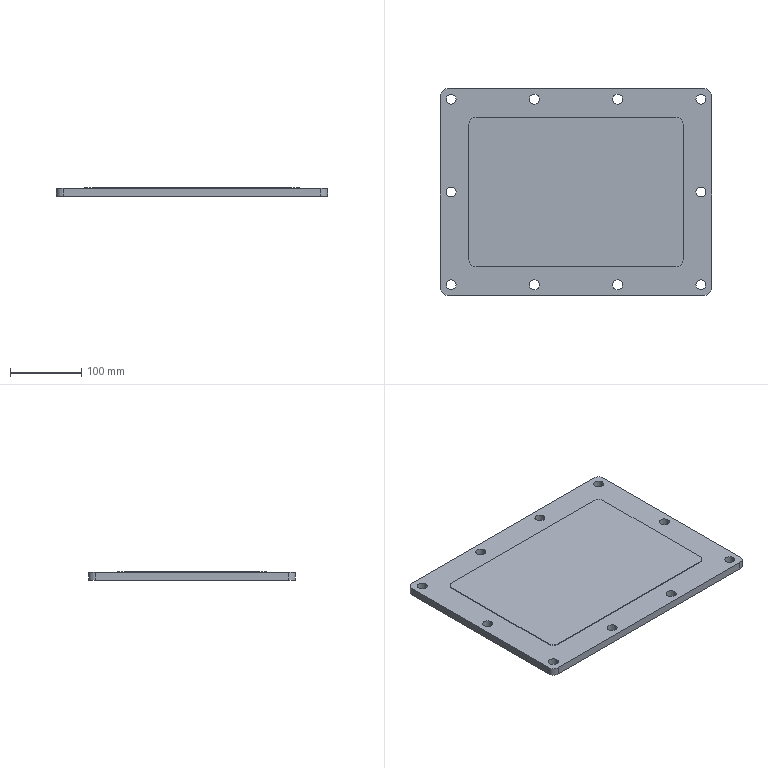Part | SolidWorks | features Extrusion 1, ICE 1 | 1 solid | 39 faces | box 380 x 290 x 12 mm | volume 1257237 mm3 | cylinder 28 | plane 11 | commonest cylinder face diameters 14 x20 20 x8
STEP:
#1=CARTESIAN_POINT('',(8.,145.,11.));
#2=VERTEX_POINT('',#1);
#3=CARTESIAN_POINT('',(22.,145.,11.));
#4=VERTEX_POINT('',#3);
#5=CARTESIAN_POINT('',(15.,145.,11.));
#6=DIRECTION('',(0.,0.,1.));
#7=DIRECTION('',(1.,0.,0.));
#8=AXIS2_PLACEMENT_3D('',#5,#6,#7);
#9=CIRCLE('',#8,7.);
#10=EDGE_CURVE('',#2,#4,#9,.T.);
#11=ORIENTED_EDGE('',*,*,#10,.T.);
#12=CARTESIAN_POINT('',(22.,145.,0.));
#13=VERTEX_POINT('',#12);
#14=CARTESIAN_POINT('',(22.,145.,12.));
#15=DIRECTION('',(0.,0.,-1.));
#16=VECTOR('',#15,1000.);
#17=LINE('',#14,#16);
#18=EDGE_CURVE('',#4,#13,#17,.T.);
#19=ORIENTED_EDGE('',*,*,#18,.T.);
#20=CARTESIAN_POINT('',(8.,145.,0.));
#21=VERTEX_POINT('',#20);
#22=CARTESIAN_POINT('',(15.,145.,0.));
#23=DIRECTION('',(0.,0.,1.));
#24=DIRECTION('',(1.,0.,0.));
#25=AXIS2_PLACEMENT_3D('',#22,#23,#24);
#26=CIRCLE('',#25,7.);
#27=EDGE_CURVE('',#21,#13,#26,.T.);
#28=ORIENTED_EDGE('',*,*,#27,.F.);
#29=CARTESIAN_POINT('',(8.,145.,12.));
#30=DIRECTION('',(0.,0.,-1.));
#31=VECTOR('',#30,1000.);
#32=LINE('',#29,#31);
#33=EDGE_CURVE('',#2,#21,#32,.T.);
#34=ORIENTED_EDGE('',*,*,#33,.F.);
#35=EDGE_LOOP('',(#11,#19,#28,#34));
#36=FACE_OUTER_BOUND('',#35,.T.);
#37=CARTESIAN_POINT('',(15.,145.,12.));
#38=DIRECTION('',(0.,0.,-1.));
#39=DIRECTION('',(-1.,0.,0.));
#40=AXIS2_PLACEMENT_3D('',#37,#38,#39);
#41=CYLINDRICAL_SURFACE('',#40,7.);
#42=ADVANCED_FACE('',(#36),#41,.F.);
#43=CARTESIAN_POINT('',(8.,15.,11.));
#44=VERTEX_POINT('',#43);
#45=CARTESIAN_POINT('',(22.,15.,11.));
#46=VERTEX_POINT('',#45);
#47=CARTESIAN_POINT('',(15.,15.,11.));
#48=DIRECTION('',(0.,0.,1.));
#49=DIRECTION('',(1.,0.,0.));
#50=AXIS2_PLACEMENT_3D('',#47,#48,#49);
#51=CIRCLE('',#50,7.);
#52=EDGE_CURVE('',#44,#46,#51,.T.);
#53=ORIENTED_EDGE('',*,*,#52,.T.);
#54=CARTESIAN_POINT('',(22.,15.,0.));
#55=VERTEX_POINT('',#54);
#56=CARTESIAN_POINT('',(22.,15.,12.));
#57=DIRECTION('',(0.,0.,-1.));
#58=VECTOR('',#57,1000.);
#59=LINE('',#56,#58);
#60=EDGE_CURVE('',#46,#55,#59,.T.);
#61=ORIENTED_EDGE('',*,*,#60,.T.);
#62=CARTESIAN_POINT('',(8.,15.,0.));
#63=VERTEX_POINT('',#62);
#64=CARTESIAN_POINT('',(15.,15.,0.));
#65=DIRECTION('',(0.,0.,1.));
#66=DIRECTION('',(1.,0.,0.));
#67=AXIS2_PLACEMENT_3D('',#64,#65,#66);
#68=CIRCLE('',#67,7.);
#69=EDGE_CURVE('',#63,#55,#68,.T.);
#70=ORIENTED_EDGE('',*,*,#69,.F.);
#71=CARTESIAN_POINT('',(8.,15.,12.));
#72=DIRECTION('',(0.,0.,-1.));
#73=VECTOR('',#72,1000.);
#74=LINE('',#71,#73);
#75=EDGE_CURVE('',#44,#63,#74,.T.);
#76=ORIENTED_EDGE('',*,*,#75,.F.);
#77=EDGE_LOOP('',(#53,#61,#70,#76));
#78=FACE_OUTER_BOUND('',#77,.T.);
#79=CARTESIAN_POINT('',(15.,15.,12.));
#80=DIRECTION('',(0.,0.,-1.));
#81=DIRECTION('',(-1.,0.,0.));
#82=AXIS2_PLACEMENT_3D('',#79,#80,#81);
#83=CYLINDRICAL_SURFACE('',#82,7.);
#84=ADVANCED_FACE('',(#78),#83,.F.);
#85=CARTESIAN_POINT('',(124.5,15.,11.));
#86=VERTEX_POINT('',#85);
#87=CARTESIAN_POINT('',(138.5,15.,11.));
#88=VERTEX_POINT('',#87);
#89=CARTESIAN_POINT('',(131.5,15.,11.));
#90=DIRECTION('',(0.,0.,1.));
#91=DIRECTION('',(1.,0.,0.));
#92=AXIS2_PLACEMENT_3D('',#89,#90,#91);
#93=CIRCLE('',#92,7.);
#94=EDGE_CURVE('',#86,#88,#93,.T.);
#95=ORIENTED_EDGE('',*,*,#94,.T.);
#96=CARTESIAN_POINT('',(138.5,15.,0.));
#97=VERTEX_POINT('',#96);
#98=CARTESIAN_POINT('',(138.5,15.,12.));
#99=DIRECTION('',(0.,0.,-1.));
#100=VECTOR('',#99,1000.);
#101=LINE('',#98,#100);
#102=EDGE_CURVE('',#88,#97,#101,.T.);
#103=ORIENTED_EDGE('',*,*,#102,.T.);
#104=CARTESIAN_POINT('',(124.5,15.,0.));
#105=VERTEX_POINT('',#104);
#106=CARTESIAN_POINT('',(131.5,15.,0.));
#107=DIRECTION('',(0.,0.,1.));
#108=DIRECTION('',(1.,0.,0.));
#109=AXIS2_PLACEMENT_3D('',#106,#107,#108);
#110=CIRCLE('',#109,7.);
#111=EDGE_CURVE('',#105,#97,#110,.T.);
#112=ORIENTED_EDGE('',*,*,#111,.F.);
#113=CARTESIAN_POINT('',(124.5,15.,12.));
#114=DIRECTION('',(0.,0.,-1.));
#115=VECTOR('',#114,1000.);
#116=LINE('',#113,#115);
#117=EDGE_CURVE('',#86,#105,#116,.T.);
#118=ORIENTED_EDGE('',*,*,#117,.F.);
#119=EDGE_LOOP('',(#95,#103,#112,#118));
#120=FACE_OUTER_BOUND('',#119,.T.);
#121=CARTESIAN_POINT('',(131.5,15.,12.));
#122=DIRECTION('',(0.,0.,-1.));
#123=DIRECTION('',(-1.,0.,0.));
#124=AXIS2_PLACEMENT_3D('',#121,#122,#123);
#125=CYLINDRICAL_SURFACE('',#124,7.);
#126=ADVANCED_FACE('',(#120),#125,.F.);
#127=CARTESIAN_POINT('',(241.5,15.,11.));
#128=VERTEX_POINT('',#127);
#129=CARTESIAN_POINT('',(255.5,15.,11.));
#130=VERTEX_POINT('',#129);
#131=CARTESIAN_POINT('',(248.5,15.,11.));
#132=DIRECTION('',(0.,0.,1.));
#133=DIRECTION('',(1.,0.,0.));
#134=AXIS2_PLACEMENT_3D('',#131,#132,#133);
#135=CIRCLE('',#134,7.);
#136=EDGE_CURVE('',#128,#130,#135,.T.);
#137=ORIENTED_EDGE('',*,*,#136,.T.);
#138=CARTESIAN_POINT('',(255.5,15.,0.));
#139=VERTEX_POINT('',#138);
#140=CARTESIAN_POINT('',(255.5,15.,12.));
#141=DIRECTION('',(0.,0.,-1.));
#142=VECTOR('',#141,1000.);
#143=LINE('',#140,#142);
#144=EDGE_CURVE('',#130,#139,#143,.T.);
#145=ORIENTED_EDGE('',*,*,#144,.T.);
#146=CARTESIAN_POINT('',(241.5,15.,0.));
#147=VERTEX_POINT('',#146);
#148=CARTESIAN_POINT('',(248.5,15.,0.));
#149=DIRECTION('',(0.,0.,1.));
#150=DIRECTION('',(1.,0.,0.));
#151=AXIS2_PLACEMENT_3D('',#148,#149,#150);
#152=CIRCLE('',#151,7.);
#153=EDGE_CURVE('',#147,#139,#152,.T.);
#154=ORIENTED_EDGE('',*,*,#153,.F.);
#155=CARTESIAN_POINT('',(241.5,15.,12.));
#156=DIRECTION('',(0.,0.,-1.));
#157=VECTOR('',#156,1000.);
#158=LINE('',#155,#157);
#159=EDGE_CURVE('',#128,#147,#158,.T.);
#160=ORIENTED_EDGE('',*,*,#159,.F.);
#161=EDGE_LOOP('',(#137,#145,#154,#160));
#162=FACE_OUTER_BOUND('',#161,.T.);
#163=CARTESIAN_POINT('',(248.5,15.,12.));
#164=DIRECTION('',(0.,0.,-1.));
#165=DIRECTION('',(-1.,0.,0.));
#166=AXIS2_PLACEMENT_3D('',#163,#164,#165);
#167=CYLINDRICAL_SURFACE('',#166,7.);
#168=ADVANCED_FACE('',(#162),#167,.F.);
#169=CARTESIAN_POINT('',(358.,15.,11.));
#170=VERTEX_POINT('',#169);
#171=CARTESIAN_POINT('',(372.,15.,11.));
#172=VERTEX_POINT('',#171);
#173=CARTESIAN_POINT('',(365.,15.,11.));
#174=DIRECTION('',(0.,0.,1.));
#175=DIRECTION('',(1.,0.,0.));
#176=AXIS2_PLACEMENT_3D('',#173,#174,#175);
#177=CIRCLE('',#176,7.);
#178=EDGE_CURVE('',#170,#172,#177,.T.);
#179=ORIENTED_EDGE('',*,*,#178,.T.);
#180=CARTESIAN_POINT('',(372.,15.,0.));
#181=VERTEX_POINT('',#180);
#182=CARTESIAN_POINT('',(372.,15.,12.));
#183=DIRECTION('',(0.,0.,-1.));
#184=VECTOR('',#183,1000.);
#185=LINE('',#182,#184);
#186=EDGE_CURVE('',#172,#181,#185,.T.);
#187=ORIENTED_EDGE('',*,*,#186,.T.);
#188=CARTESIAN_POINT('',(358.,15.,0.));
#189=VERTEX_POINT('',#188);
#190=CARTESIAN_POINT('',(365.,15.,0.));
#191=DIRECTION('',(0.,0.,1.));
#192=DIRECTION('',(1.,0.,0.));
#193=AXIS2_PLACEMENT_3D('',#190,#191,#192);
#194=CIRCLE('',#193,7.);
#195=EDGE_CURVE('',#189,#181,#194,.T.);
#196=ORIENTED_EDGE('',*,*,#195,.F.);
#197=CARTESIAN_POINT('',(358.,15.,12.));
#198=DIRECTION('',(0.,0.,-1.));
#199=VECTOR('',#198,1000.);
#200=LINE('',#197,#199);
#201=EDGE_CURVE('',#170,#189,#200,.T.);
#202=ORIENTED_EDGE('',*,*,#201,.F.);
#203=EDGE_LOOP('',(#179,#187,#196,#202));
#204=FACE_OUTER_BOUND('',#203,.T.);
#205=CARTESIAN_POINT('',(365.,15.,12.));
#206=DIRECTION('',(0.,0.,-1.));
#207=DIRECTION('',(-1.,0.,0.));
#208=AXIS2_PLACEMENT_3D('',#205,#206,#207);
#209=CYLINDRICAL_SURFACE('',#208,7.);
#210=ADVANCED_FACE('',(#204),#209,.F.);
#211=CARTESIAN_POINT('',(358.,145.,11.));
#212=VERTEX_POINT('',#211);
#213=CARTESIAN_POINT('',(372.,145.,11.));
#214=VERTEX_POINT('',#213);
#215=CARTESIAN_POINT('',(365.,145.,11.));
#216=DIRECTION('',(0.,0.,1.));
#217=DIRECTION('',(1.,0.,0.));
#218=AXIS2_PLACEMENT_3D('',#215,#216,#217);
#219=CIRCLE('',#218,7.);
#220=EDGE_CURVE('',#212,#214,#219,.T.);
#221=ORIENTED_EDGE('',*,*,#220,.T.);
#222=CARTESIAN_POINT('',(372.,145.,0.));
#223=VERTEX_POINT('',#222);
#224=CARTESIAN_POINT('',(372.,145.,12.));
#225=DIRECTION('',(0.,0.,-1.));
#226=VECTOR('',#225,1000.);
#227=LINE('',#224,#226);
#228=EDGE_CURVE('',#214,#223,#227,.T.);
#229=ORIENTED_EDGE('',*,*,#228,.T.);
#230=CARTESIAN_POINT('',(358.,145.,0.));
#231=VERTEX_POINT('',#230);
#232=CARTESIAN_POINT('',(365.,145.,0.));
#233=DIRECTION('',(0.,0.,1.));
#234=DIRECTION('',(1.,0.,0.));
#235=AXIS2_PLACEMENT_3D('',#232,#233,#234);
#236=CIRCLE('',#235,7.);
#237=EDGE_CURVE('',#231,#223,#236,.T.);
#238=ORIENTED_EDGE('',*,*,#237,.F.);
#239=CARTESIAN_POINT('',(358.,145.,12.));
#240=DIRECTION('',(0.,0.,-1.));
#241=VECTOR('',#240,1000.);
#242=LINE('',#239,#241);
#243=EDGE_CURVE('',#212,#231,#242,.T.);
#244=ORIENTED_EDGE('',*,*,#243,.F.);
#245=EDGE_LOOP('',(#221,#229,#238,#244));
#246=FACE_OUTER_BOUND('',#245,.T.);
#247=CARTESIAN_POINT('',(365.,145.,12.));
#248=DIRECTION('',(0.,0.,-1.));
#249=DIRECTION('',(-1.,0.,0.));
#250=AXIS2_PLACEMENT_3D('',#247,#248,#249);
#251=CYLINDRICAL_SURFACE('',#250,7.);
#252=ADVANCED_FACE('',(#246),#251,.F.);
#253=CARTESIAN_POINT('',(358.,275.,11.));
#254=VERTEX_POINT('',#253);
#255=CARTESIAN_POINT('',(372.,275.,11.));
#256=VERTEX_POINT('',#255);
#257=CARTESIAN_POINT('',(365.,275.,11.));
#258=DIRECTION('',(0.,0.,1.));
#259=DIRECTION('',(1.,0.,0.));
#260=AXIS2_PLACEMENT_3D('',#257,#258,#259);
#261=CIRCLE('',#260,7.);
#262=EDGE_CURVE('',#254,#256,#261,.T.);
#263=ORIENTED_EDGE('',*,*,#262,.T.);
#264=CARTESIAN_POINT('',(372.,275.,0.));
#265=VERTEX_POINT('',#264);
#266=CARTESIAN_POINT('',(372.,275.,12.));
#267=DIRECTION('',(0.,0.,-1.));
#268=VECTOR('',#267,1000.);
#269=LINE('',#266,#268);
#270=EDGE_CURVE('',#256,#265,#269,.T.);
#271=ORIENTED_EDGE('',*,*,#270,.T.);
#272=CARTESIAN_POINT('',(358.,275.,0.));
#273=VERTEX_POINT('',#272);
#274=CARTESIAN_POINT('',(365.,275.,0.));
#275=DIRECTION('',(0.,0.,1.));
#276=DIRECTION('',(1.,0.,0.));
#277=AXIS2_PLACEMENT_3D('',#274,#275,#276);
#278=CIRCLE('',#277,7.);
#279=EDGE_CURVE('',#273,#265,#278,.T.);
#280=ORIENTED_EDGE('',*,*,#279,.F.);
#281=CARTESIAN_POINT('',(358.,275.,12.));
#282=DIRECTION('',(0.,0.,-1.));
#283=VECTOR('',#282,1000.);
#284=LINE('',#281,#283);
#285=EDGE_CURVE('',#254,#273,#284,.T.);
#286=ORIENTED_EDGE('',*,*,#285,.F.);
#287=EDGE_LOOP('',(#263,#271,#280,#286));
#288=FACE_OUTER_BOUND('',#287,.T.);
#289=CARTESIAN_POINT('',(365.,275.,12.));
#290=DIRECTION('',(0.,0.,-1.));
#291=DIRECTION('',(-1.,0.,0.));
#292=AXIS2_PLACEMENT_3D('',#289,#290,#291);
#293=CYLINDRICAL_SURFACE('',#292,7.);
#294=ADVANCED_FACE('',(#288),#293,.F.);
#295=CARTESIAN_POINT('',(241.5,275.,11.));
#296=VERTEX_POINT('',#295);
#297=CARTESIAN_POINT('',(255.5,275.,11.));
#298=VERTEX_POINT('',#297);
#299=CARTESIAN_POINT('',(248.5,275.,11.));
#300=DIRECTION('',(0.,0.,1.));
#301=DIRECTION('',(1.,0.,0.));
#302=AXIS2_PLACEMENT_3D('',#299,#300,#301);
#303=CIRCLE('',#302,7.);
#304=EDGE_CURVE('',#296,#298,#303,.T.);
#305=ORIENTED_EDGE('',*,*,#304,.T.);
#306=CARTESIAN_POINT('',(255.5,275.,0.));
#307=VERTEX_POINT('',#306);
#308=CARTESIAN_POINT('',(255.5,275.,12.));
#309=DIRECTION('',(0.,0.,-1.));
#310=VECTOR('',#309,1000.);
#311=LINE('',#308,#310);
#312=EDGE_CURVE('',#298,#307,#311,.T.);
#313=ORIENTED_EDGE('',*,*,#312,.T.);
#314=CARTESIAN_POINT('',(241.5,275.,0.));
#315=VERTEX_POINT('',#314);
#316=CARTESIAN_POINT('',(248.5,275.,0.));
#317=DIRECTION('',(0.,0.,1.));
#318=DIRECTION('',(1.,0.,0.));
#319=AXIS2_PLACEMENT_3D('',#316,#317,#318);
#320=CIRCLE('',#319,7.);
#321=EDGE_CURVE('',#315,#307,#320,.T.);
#322=ORIENTED_EDGE('',*,*,#321,.F.);
#323=CARTESIAN_POINT('',(241.5,275.,12.));
#324=DIRECTION('',(0.,0.,-1.));
#325=VECTOR('',#324,1000.);
#326=LINE('',#323,#325);
#327=EDGE_CURVE('',#296,#315,#326,.T.);
#328=ORIENTED_EDGE('',*,*,#327,.F.);
#329=EDGE_LOOP('',(#305,#313,#322,#328));
#330=FACE_OUTER_BOUND('',#329,.T.);
#331=CARTESIAN_POINT('',(248.5,275.,12.));
#332=DIRECTION('',(0.,0.,-1.));
#333=DIRECTION('',(-1.,0.,0.));
#334=AXIS2_PLACEMENT_3D('',#331,#332,#333);
#335=CYLINDRICAL_SURFACE('',#334,7.);
#336=ADVANCED_FACE('',(#330),#335,.F.);
#337=CARTESIAN_POINT('',(124.5,275.,11.));
#338=VERTEX_POINT('',#337);
#339=CARTESIAN_POINT('',(138.5,275.,11.));
#340=VERTEX_POINT('',#339);
#341=CARTESIAN_POINT('',(131.5,275.,11.));
#342=DIRECTION('',(0.,0.,1.));
#343=DIRECTION('',(1.,0.,0.));
#344=AXIS2_PLACEMENT_3D('',#341,#342,#343);
#345=CIRCLE('',#344,7.);
#346=EDGE_CURVE('',#338,#340,#345,.T.);
#347=ORIENTED_EDGE('',*,*,#346,.T.);
#348=CARTESIAN_POINT('',(138.5,275.,0.));
#349=VERTEX_POINT('',#348);
#350=CARTESIAN_POINT('',(138.5,275.,12.));
#351=DIRECTION('',(0.,0.,-1.));
#352=VECTOR('',#351,1000.);
#353=LINE('',#350,#352);
#354=EDGE_CURVE('',#340,#349,#353,.T.);
#355=ORIENTED_EDGE('',*,*,#354,.T.);
#356=CARTESIAN_POINT('',(124.5,275.,0.));
#357=VERTEX_POINT('',#356);
#358=CARTESIAN_POINT('',(131.5,275.,0.));
#359=DIRECTION('',(0.,0.,1.));
#360=DIRECTION('',(1.,0.,0.));
#361=AXIS2_PLACEMENT_3D('',#358,#359,#360);
#362=CIRCLE('',#361,7.);
#363=EDGE_CURVE('',#357,#349,#362,.T.);
#364=ORIENTED_EDGE('',*,*,#363,.F.);
#365=CARTESIAN_POINT('',(124.5,275.,12.));
#366=DIRECTION('',(0.,0.,-1.));
#367=VECTOR('',#366,1000.);
#368=LINE('',#365,#367);
#369=EDGE_CURVE('',#338,#357,#368,.T.);
#370=ORIENTED_EDGE('',*,*,#369,.F.);
#371=EDGE_LOOP('',(#347,#355,#364,#370));
#372=FACE_OUTER_BOUND('',#371,.T.);
#373=CARTESIAN_POINT('',(131.5,275.,12.));
#374=DIRECTION('',(0.,0.,-1.));
#375=DIRECTION('',(-1.,0.,0.));
#376=AXIS2_PLACEMENT_3D('',#373,#374,#375);
#377=CYLINDRICAL_SURFACE('',#376,7.);
#378=ADVANCED_FACE('',(#372),#377,.F.);
#379=CARTESIAN_POINT('',(8.,275.,11.));
#380=VERTEX_POINT('',#379);
#381=CARTESIAN_POINT('',(22.,275.,11.));
#382=VERTEX_POINT('',#381);
#383=CARTESIAN_POINT('',(15.,275.,11.));
#384=DIRECTION('',(0.,0.,1.));
#385=DIRECTION('',(1.,0.,0.));
#386=AXIS2_PLACEMENT_3D('',#383,#384,#385);
#387=CIRCLE('',#386,7.);
#388=EDGE_CURVE('',#380,#382,#387,.T.);
#389=ORIENTED_EDGE('',*,*,#388,.T.);
#390=CARTESIAN_POINT('',(22.,275.,0.));
#391=VERTEX_POINT('',#390);
#392=CARTESIAN_POINT('',(22.,275.,12.));
#393=DIRECTION('',(0.,0.,-1.));
#394=VECTOR('',#393,1000.);
#395=LINE('',#392,#394);
#396=EDGE_CURVE('',#382,#391,#395,.T.);
#397=ORIENTED_EDGE('',*,*,#396,.T.);
#398=CARTESIAN_POINT('',(8.,275.,0.));
#399=VERTEX_POINT('',#398);
#400=CARTESIAN_POINT('',(15.,275.,0.));
#401=DIRECTION('',(0.,0.,1.));
#402=DIRECTION('',(1.,0.,0.));
#403=AXIS2_PLACEMENT_3D('',#400,#401,#402);
#404=CIRCLE('',#403,7.);
#405=EDGE_CURVE('',#399,#391,#404,.T.);
#406=ORIENTED_EDGE('',*,*,#405,.F.);
#407=CARTESIAN_POINT('',(8.,275.,12.));
#408=DIRECTION('',(0.,0.,-1.));
#409=VECTOR('',#408,1000.);
#410=LINE('',#407,#409);
#411=EDGE_CURVE('',#380,#399,#410,.T.);
#412=ORIENTED_EDGE('',*,*,#411,.F.);
#413=EDGE_LOOP('',(#389,#397,#406,#412));
#414=FACE_OUTER_BOUND('',#413,.T.);
#415=CARTESIAN_POINT('',(15.,275.,12.));
#416=DIRECTION('',(0.,0.,-1.));
#417=DIRECTION('',(-1.,0.,0.));
#418=AXIS2_PLACEMENT_3D('',#415,#416,#417);
#419=CYLINDRICAL_SURFACE('',#418,7.);
#420=ADVANCED_FACE('',(#414),#419,.F.);
#421=CARTESIAN_POINT('',(0.,10.,11.));
#422=VERTEX_POINT('',#421);
#423=CARTESIAN_POINT('',(10.,0.,11.));
#424=VERTEX_POINT('',#423);
#425=CARTESIAN_POINT('',(10.,10.,11.));
#426=DIRECTION('',(0.,0.,1.));
#427=DIRECTION('',(1.,0.,0.));
#428=AXIS2_PLACEMENT_3D('',#425,#426,#427);
#429=CIRCLE('',#428,10.);
#430=EDGE_CURVE('',#422,#424,#429,.T.);
#431=ORIENTED_EDGE('',*,*,#430,.F.);
#432=CARTESIAN_POINT('',(0.,10.,0.));
#433=VERTEX_POINT('',#432);
#434=CARTESIAN_POINT('',(0.,10.,12.));
#435=DIRECTION('',(0.,0.,-1.));
#436=VECTOR('',#435,1000.);
#437=LINE('',#434,#436);
#438=EDGE_CURVE('',#422,#433,#437,.T.);
#439=ORIENTED_EDGE('',*,*,#438,.T.);
#440=CARTESIAN_POINT('',(10.,0.,0.));
#441=VERTEX_POINT('',#440);
#442=CARTESIAN_POINT('',(10.,10.,0.));
#443=DIRECTION('',(0.,0.,1.));
#444=DIRECTION('',(-1.,0.,0.));
#445=AXIS2_PLACEMENT_3D('',#442,#443,#444);
#446=CIRCLE('',#445,10.);
#447=EDGE_CURVE('',#433,#441,#446,.T.);
#448=ORIENTED_EDGE('',*,*,#447,.T.);
#449=CARTESIAN_POINT('',(10.,0.,12.));
#450=DIRECTION('',(0.,0.,-1.));
#451=VECTOR('',#450,1000.);
#452=LINE('',#449,#451);
#453=EDGE_CURVE('',#424,#441,#452,.T.);
#454=ORIENTED_EDGE('',*,*,#453,.F.);
#455=EDGE_LOOP('',(#431,#439,#448,#454));
#456=FACE_OUTER_BOUND('',#455,.T.);
#457=CARTESIAN_POINT('',(10.,10.,12.));
#458=DIRECTION('',(0.,0.,-1.));
#459=DIRECTION('',(-1.,0.,0.));
#460=AXIS2_PLACEMENT_3D('',#457,#458,#459);
#461=CYLINDRICAL_SURFACE('',#460,10.);
#462=ADVANCED_FACE('',(#456),#461,.T.);
#463=CARTESIAN_POINT('',(370.,0.,11.));
#464=VERTEX_POINT('',#463);
#465=CARTESIAN_POINT('',(10.,0.,11.));
#466=DIRECTION('',(1.,0.,0.));
#467=VECTOR('',#466,1000.);
#468=LINE('',#465,#467);
#469=EDGE_CURVE('',#424,#464,#468,.T.);
#470=ORIENTED_EDGE('',*,*,#469,.F.);
#471=ORIENTED_EDGE('',*,*,#453,.T.);
#472=CARTESIAN_POINT('',(370.,0.,0.));
#473=VERTEX_POINT('',#472);
#474=CARTESIAN_POINT('',(10.,0.,0.));
#475=DIRECTION('',(1.,0.,0.));
#476=VECTOR('',#475,1000.);
#477=LINE('',#474,#476);
#478=EDGE_CURVE('',#441,#473,#477,.T.);
#479=ORIENTED_EDGE('',*,*,#478,.T.);
#480=CARTESIAN_POINT('',(370.,0.,12.));
#481=DIRECTION('',(0.,0.,-1.));
#482=VECTOR('',#481,1000.);
#483=LINE('',#480,#482);
#484=EDGE_CURVE('',#464,#473,#483,.T.);
#485=ORIENTED_EDGE('',*,*,#484,.F.);
#486=EDGE_LOOP('',(#470,#471,#479,#485));
#487=FACE_OUTER_BOUND('',#486,.T.);
#488=CARTESIAN_POINT('',(10.,0.,12.));
#489=DIRECTION('',(0.,1.,0.));
#490=DIRECTION('',(0.,0.,1.));
#491=AXIS2_PLACEMENT_3D('',#488,#489,#490);
#492=PLANE('',#491);
#493=ADVANCED_FACE('',(#487),#492,.F.);
#494=CARTESIAN_POINT('',(380.,10.,11.));
#495=VERTEX_POINT('',#494);
#496=CARTESIAN_POINT('',(370.,10.,11.));
#497=DIRECTION('',(0.,0.,1.));
#498=DIRECTION('',(1.,0.,0.));
#499=AXIS2_PLACEMENT_3D('',#496,#497,#498);
#500=CIRCLE('',#499,10.);
#501=EDGE_CURVE('',#464,#495,#500,.T.);
#502=ORIENTED_EDGE('',*,*,#501,.F.);
#503=ORIENTED_EDGE('',*,*,#484,.T.);
#504=CARTESIAN_POINT('',(380.,10.,0.));
#505=VERTEX_POINT('',#504);
#506=CARTESIAN_POINT('',(370.,10.,0.));
#507=DIRECTION('',(0.,0.,1.));
#508=DIRECTION('',(1.,0.,0.));
#509=AXIS2_PLACEMENT_3D('',#506,#507,#508);
#510=CIRCLE('',#509,10.);
#511=EDGE_CURVE('',#473,#505,#510,.T.);
#512=ORIENTED_EDGE('',*,*,#511,.T.);
#513=CARTESIAN_POINT('',(380.,10.,12.));
#514=DIRECTION('',(0.,0.,-1.));
#515=VECTOR('',#514,1000.);
#516=LINE('',#513,#515);
#517=EDGE_CURVE('',#495,#505,#516,.T.);
#518=ORIENTED_EDGE('',*,*,#517,.F.);
#519=EDGE_LOOP('',(#502,#503,#512,#518));
#520=FACE_OUTER_BOUND('',#519,.T.);
#521=CARTESIAN_POINT('',(370.,10.,12.));
#522=DIRECTION('',(0.,0.,-1.));
#523=DIRECTION('',(-1.,0.,0.));
#524=AXIS2_PLACEMENT_3D('',#521,#522,#523);
#525=CYLINDRICAL_SURFACE('',#524,10.);
#526=ADVANCED_FACE('',(#520),#525,.T.);
#527=CARTESIAN_POINT('',(380.,280.,11.));
#528=VERTEX_POINT('',#527);
#529=CARTESIAN_POINT('',(380.,10.,11.));
#530=DIRECTION('',(0.,1.,0.));
#531=VECTOR('',#530,1000.);
#532=LINE('',#529,#531);
#533=EDGE_CURVE('',#495,#528,#532,.T.);
#534=ORIENTED_EDGE('',*,*,#533,.F.);
#535=ORIENTED_EDGE('',*,*,#517,.T.);
#536=CARTESIAN_POINT('',(380.,280.,0.));
#537=VERTEX_POINT('',#536);
#538=CARTESIAN_POINT('',(380.,10.,0.));
#539=DIRECTION('',(0.,1.,0.));
#540=VECTOR('',#539,1000.);
#541=LINE('',#538,#540);
#542=EDGE_CURVE('',#505,#537,#541,.T.);
#543=ORIENTED_EDGE('',*,*,#542,.T.);
#544=CARTESIAN_POINT('',(380.,280.,12.));
#545=DIRECTION('',(0.,0.,-1.));
#546=VECTOR('',#545,1000.);
#547=LINE('',#544,#546);
#548=EDGE_CURVE('',#528,#537,#547,.T.);
#549=ORIENTED_EDGE('',*,*,#548,.F.);
#550=EDGE_LOOP('',(#534,#535,#543,#549));
#551=FACE_OUTER_BOUND('',#550,.T.);
#552=CARTESIAN_POINT('',(380.,10.,12.));
#553=DIRECTION('',(-1.,0.,0.));
#554=DIRECTION('',(0.,0.,1.));
#555=AXIS2_PLACEMENT_3D('',#552,#553,#554);
#556=PLANE('',#555);
#557=ADVANCED_FACE('',(#551),#556,.F.);
#558=CARTESIAN_POINT('',(370.,290.,11.));
#559=VERTEX_POINT('',#558);
#560=CARTESIAN_POINT('',(370.,280.,11.));
#561=DIRECTION('',(0.,0.,1.));
#562=DIRECTION('',(1.,0.,0.));
#563=AXIS2_PLACEMENT_3D('',#560,#561,#562);
#564=CIRCLE('',#563,10.);
#565=EDGE_CURVE('',#528,#559,#564,.T.);
#566=ORIENTED_EDGE('',*,*,#565,.F.);
#567=ORIENTED_EDGE('',*,*,#548,.T.);
#568=CARTESIAN_POINT('',(370.,290.,0.));
#569=VERTEX_POINT('',#568);
#570=CARTESIAN_POINT('',(370.,280.,0.));
#571=DIRECTION('',(0.,0.,1.));
#572=DIRECTION('',(-1.,0.,0.));
#573=AXIS2_PLACEMENT_3D('',#570,#571,#572);
#574=CIRCLE('',#573,10.);
#575=EDGE_CURVE('',#537,#569,#574,.T.);
#576=ORIENTED_EDGE('',*,*,#575,.T.);
#577=CARTESIAN_POINT('',(370.,290.,12.));
#578=DIRECTION('',(0.,0.,-1.));
#579=VECTOR('',#578,1000.);
#580=LINE('',#577,#579);
#581=EDGE_CURVE('',#559,#569,#580,.T.);
#582=ORIENTED_EDGE('',*,*,#581,.F.);
#583=EDGE_LOOP('',(#566,#567,#576,#582));
#584=FACE_OUTER_BOUND('',#583,.T.);
#585=CARTESIAN_POINT('',(370.,280.,12.));
#586=DIRECTION('',(0.,0.,-1.));
#587=DIRECTION('',(-1.,0.,0.));
#588=AXIS2_PLACEMENT_3D('',#585,#586,#587);
#589=CYLINDRICAL_SURFACE('',#588,10.);
#590=ADVANCED_FACE('',(#584),#589,.T.);
#591=CARTESIAN_POINT('',(10.,290.,11.));
#592=VERTEX_POINT('',#591);
#593=CARTESIAN_POINT('',(10.,290.,11.));
#594=DIRECTION('',(-1.,0.,0.));
#595=VECTOR('',#594,1000.);
#596=LINE('',#593,#595);
#597=EDGE_CURVE('',#559,#592,#596,.T.);
#598=ORIENTED_EDGE('',*,*,#597,.F.);
#599=ORIENTED_EDGE('',*,*,#581,.T.);
#600=CARTESIAN_POINT('',(10.,290.,0.));
#601=VERTEX_POINT('',#600);
#602=CARTESIAN_POINT('',(10.,290.,0.));
#603=DIRECTION('',(-1.,0.,0.));
#604=VECTOR('',#603,1000.);
#605=LINE('',#602,#604);
#606=EDGE_CURVE('',#569,#601,#605,.T.);
#607=ORIENTED_EDGE('',*,*,#606,.T.);
#608=CARTESIAN_POINT('',(10.,290.,12.));
#609=DIRECTION('',(0.,0.,-1.));
#610=VECTOR('',#609,1000.);
#611=LINE('',#608,#610);
#612=EDGE_CURVE('',#592,#601,#611,.T.);
#613=ORIENTED_EDGE('',*,*,#612,.F.);
#614=EDGE_LOOP('',(#598,#599,#607,#613));
#615=FACE_OUTER_BOUND('',#614,.T.);
#616=CARTESIAN_POINT('',(10.,290.,12.));
#617=DIRECTION('',(0.,-1.,0.));
#618=DIRECTION('',(0.,0.,-1.));
#619=AXIS2_PLACEMENT_3D('',#616,#617,#618);
#620=PLANE('',#619);
#621=ADVANCED_FACE('',(#615),#620,.F.);
#622=CARTESIAN_POINT('',(0.,280.,11.));
#623=VERTEX_POINT('',#622);
#624=CARTESIAN_POINT('',(10.,280.,11.));
#625=DIRECTION('',(0.,0.,1.));
#626=DIRECTION('',(1.,0.,0.));
#627=AXIS2_PLACEMENT_3D('',#624,#625,#626);
#628=CIRCLE('',#627,10.);
#629=EDGE_CURVE('',#592,#623,#628,.T.);
#630=ORIENTED_EDGE('',*,*,#629,.F.);
#631=ORIENTED_EDGE('',*,*,#612,.T.);
#632=CARTESIAN_POINT('',(0.,280.,0.));
#633=VERTEX_POINT('',#632);
#634=CARTESIAN_POINT('',(10.,280.,0.));
#635=DIRECTION('',(0.,0.,1.));
#636=DIRECTION('',(-1.,0.,0.));
#637=AXIS2_PLACEMENT_3D('',#634,#635,#636);
#638=CIRCLE('',#637,10.);
#639=EDGE_CURVE('',#601,#633,#638,.T.);
#640=ORIENTED_EDGE('',*,*,#639,.T.);
#641=CARTESIAN_POINT('',(0.,280.,12.));
#642=DIRECTION('',(0.,0.,-1.));
#643=VECTOR('',#642,1000.);
#644=LINE('',#641,#643);
#645=EDGE_CURVE('',#623,#633,#644,.T.);
#646=ORIENTED_EDGE('',*,*,#645,.F.);
#647=EDGE_LOOP('',(#630,#631,#640,#646));
#648=FACE_OUTER_BOUND('',#647,.T.);
#649=CARTESIAN_POINT('',(10.,280.,12.));
#650=DIRECTION('',(0.,0.,-1.));
#651=DIRECTION('',(-1.,0.,0.));
#652=AXIS2_PLACEMENT_3D('',#649,#650,#651);
#653=CYLINDRICAL_SURFACE('',#652,10.);
#654=ADVANCED_FACE('',(#648),#653,.T.);
#655=CARTESIAN_POINT('',(0.,10.,11.));
#656=DIRECTION('',(0.,-1.,0.));
#657=VECTOR('',#656,1000.);
#658=LINE('',#655,#657);
#659=EDGE_CURVE('',#623,#422,#658,.T.);
#660=ORIENTED_EDGE('',*,*,#659,.F.);
#661=ORIENTED_EDGE('',*,*,#645,.T.);
#662=CARTESIAN_POINT('',(0.,10.,0.));
#663=DIRECTION('',(0.,-1.,0.));
#664=VECTOR('',#663,1000.);
#665=LINE('',#662,#664);
#666=EDGE_CURVE('',#633,#433,#665,.T.);
#667=ORIENTED_EDGE('',*,*,#666,.T.);
#668=ORIENTED_EDGE('',*,*,#438,.F.);
#669=EDGE_LOOP('',(#660,#661,#667,#668));
#670=FACE_OUTER_BOUND('',#669,.T.);
#671=CARTESIAN_POINT('',(0.,10.,12.));
#672=DIRECTION('',(1.,0.,0.));
#673=DIRECTION('',(0.,0.,-1.));
#674=AXIS2_PLACEMENT_3D('',#671,#672,#673);
#675=PLANE('',#674);
#676=ADVANCED_FACE('',(#670),#675,.F.);
#677=ORIENTED_EDGE('',*,*,#396,.F.);
#678=CARTESIAN_POINT('',(15.,275.,11.));
#679=DIRECTION('',(0.,0.,1.));
#680=DIRECTION('',(1.,0.,0.));
#681=AXIS2_PLACEMENT_3D('',#678,#679,#680);
#682=CIRCLE('',#681,7.);
#683=EDGE_CURVE('',#382,#380,#682,.T.);
#684=ORIENTED_EDGE('',*,*,#683,.T.);
#685=ORIENTED_EDGE('',*,*,#411,.T.);
#686=CARTESIAN_POINT('',(15.,275.,0.));
#687=DIRECTION('',(0.,0.,1.));
#688=DIRECTION('',(1.,0.,0.));
#689=AXIS2_PLACEMENT_3D('',#686,#687,#688);
#690=CIRCLE('',#689,7.);
#691=EDGE_CURVE('',#391,#399,#690,.T.);
#692=ORIENTED_EDGE('',*,*,#691,.F.);
#693=EDGE_LOOP('',(#677,#684,#685,#692));
#694=FACE_OUTER_BOUND('',#693,.T.);
#695=CARTESIAN_POINT('',(15.,275.,12.));
#696=DIRECTION('',(0.,0.,-1.));
#697=DIRECTION('',(-1.,0.,0.));
#698=AXIS2_PLACEMENT_3D('',#695,#696,#697);
#699=CYLINDRICAL_SURFACE('',#698,7.);
#700=ADVANCED_FACE('',(#694),#699,.F.);
#701=ORIENTED_EDGE('',*,*,#354,.F.);
#702=CARTESIAN_POINT('',(131.5,275.,11.));
#703=DIRECTION('',(0.,0.,1.));
#704=DIRECTION('',(1.,0.,0.));
#705=AXIS2_PLACEMENT_3D('',#702,#703,#704);
#706=CIRCLE('',#705,7.);
#707=EDGE_CURVE('',#340,#338,#706,.T.);
#708=ORIENTED_EDGE('',*,*,#707,.T.);
#709=ORIENTED_EDGE('',*,*,#369,.T.);
#710=CARTESIAN_POINT('',(131.5,275.,0.));
#711=DIRECTION('',(0.,0.,1.));
#712=DIRECTION('',(1.,0.,0.));
#713=AXIS2_PLACEMENT_3D('',#710,#711,#712);
#714=CIRCLE('',#713,7.);
#715=EDGE_CURVE('',#349,#357,#714,.T.);
#716=ORIENTED_EDGE('',*,*,#715,.F.);
#717=EDGE_LOOP('',(#701,#708,#709,#716));
#718=FACE_OUTER_BOUND('',#717,.T.);
#719=CARTESIAN_POINT('',(131.5,275.,12.));
#720=DIRECTION('',(0.,0.,-1.));
#721=DIRECTION('',(-1.,0.,0.));
#722=AXIS2_PLACEMENT_3D('',#719,#720,#721);
#723=CYLINDRICAL_SURFACE('',#722,7.);
#724=ADVANCED_FACE('',(#718),#723,.F.);
#725=ORIENTED_EDGE('',*,*,#312,.F.);
#726=CARTESIAN_POINT('',(248.5,275.,11.));
#727=DIRECTION('',(0.,0.,1.));
#728=DIRECTION('',(1.,0.,0.));
#729=AXIS2_PLACEMENT_3D('',#726,#727,#728);
#730=CIRCLE('',#729,7.);
#731=EDGE_CURVE('',#298,#296,#730,.T.);
#732=ORIENTED_EDGE('',*,*,#731,.T.);
#733=ORIENTED_EDGE('',*,*,#327,.T.);
#734=CARTESIAN_POINT('',(248.5,275.,0.));
#735=DIRECTION('',(0.,0.,1.));
#736=DIRECTION('',(1.,0.,0.));
#737=AXIS2_PLACEMENT_3D('',#734,#735,#736);
#738=CIRCLE('',#737,7.);
#739=EDGE_CURVE('',#307,#315,#738,.T.);
#740=ORIENTED_EDGE('',*,*,#739,.F.);
#741=EDGE_LOOP('',(#725,#732,#733,#740));
#742=FACE_OUTER_BOUND('',#741,.T.);
#743=CARTESIAN_POINT('',(248.5,275.,12.));
#744=DIRECTION('',(0.,0.,-1.));
#745=DIRECTION('',(-1.,0.,0.));
#746=AXIS2_PLACEMENT_3D('',#743,#744,#745);
#747=CYLINDRICAL_SURFACE('',#746,7.);
#748=ADVANCED_FACE('',(#742),#747,.F.);
#749=ORIENTED_EDGE('',*,*,#270,.F.);
#750=CARTESIAN_POINT('',(365.,275.,11.));
#751=DIRECTION('',(0.,0.,1.));
#752=DIRECTION('',(1.,0.,0.));
#753=AXIS2_PLACEMENT_3D('',#750,#751,#752);
#754=CIRCLE('',#753,7.);
#755=EDGE_CURVE('',#256,#254,#754,.T.);
#756=ORIENTED_EDGE('',*,*,#755,.T.);
#757=ORIENTED_EDGE('',*,*,#285,.T.);
#758=CARTESIAN_POINT('',(365.,275.,0.));
#759=DIRECTION('',(0.,0.,1.));
#760=DIRECTION('',(1.,0.,0.));
#761=AXIS2_PLACEMENT_3D('',#758,#759,#760);
#762=CIRCLE('',#761,7.);
#763=EDGE_CURVE('',#265,#273,#762,.T.);
#764=ORIENTED_EDGE('',*,*,#763,.F.);
#765=EDGE_LOOP('',(#749,#756,#757,#764));
#766=FACE_OUTER_BOUND('',#765,.T.);
#767=CARTESIAN_POINT('',(365.,275.,12.));
#768=DIRECTION('',(0.,0.,-1.));
#769=DIRECTION('',(-1.,0.,0.));
#770=AXIS2_PLACEMENT_3D('',#767,#768,#769);
#771=CYLINDRICAL_SURFACE('',#770,7.);
#772=ADVANCED_FACE('',(#766),#771,.F.);
#773=ORIENTED_EDGE('',*,*,#228,.F.);
#774=CARTESIAN_POINT('',(365.,145.,11.));
#775=DIRECTION('',(0.,0.,1.));
#776=DIRECTION('',(1.,0.,0.));
#777=AXIS2_PLACEMENT_3D('',#774,#775,#776);
#778=CIRCLE('',#777,7.);
#779=EDGE_CURVE('',#214,#212,#778,.T.);
#780=ORIENTED_EDGE('',*,*,#779,.T.);
#781=ORIENTED_EDGE('',*,*,#243,.T.);
#782=CARTESIAN_POINT('',(365.,145.,0.));
#783=DIRECTION('',(0.,0.,1.));
#784=DIRECTION('',(1.,0.,0.));
#785=AXIS2_PLACEMENT_3D('',#782,#783,#784);
#786=CIRCLE('',#785,7.);
#787=EDGE_CURVE('',#223,#231,#786,.T.);
#788=ORIENTED_EDGE('',*,*,#787,.F.);
#789=EDGE_LOOP('',(#773,#780,#781,#788));
#790=FACE_OUTER_BOUND('',#789,.T.);
#791=CARTESIAN_POINT('',(365.,145.,12.));
#792=DIRECTION('',(0.,0.,-1.));
#793=DIRECTION('',(-1.,0.,0.));
#794=AXIS2_PLACEMENT_3D('',#791,#792,#793);
#795=CYLINDRICAL_SURFACE('',#794,7.);
#796=ADVANCED_FACE('',(#790),#795,.F.);
#797=ORIENTED_EDGE('',*,*,#186,.F.);
#798=CARTESIAN_POINT('',(365.,15.,11.));
#799=DIRECTION('',(0.,0.,1.));
#800=DIRECTION('',(1.,0.,0.));
#801=AXIS2_PLACEMENT_3D('',#798,#799,#800);
#802=CIRCLE('',#801,7.);
#803=EDGE_CURVE('',#172,#170,#802,.T.);
#804=ORIENTED_EDGE('',*,*,#803,.T.);
#805=ORIENTED_EDGE('',*,*,#201,.T.);
#806=CARTESIAN_POINT('',(365.,15.,0.));
#807=DIRECTION('',(0.,0.,1.));
#808=DIRECTION('',(1.,0.,0.));
#809=AXIS2_PLACEMENT_3D('',#806,#807,#808);
#810=CIRCLE('',#809,7.);
#811=EDGE_CURVE('',#181,#189,#810,.T.);
#812=ORIENTED_EDGE('',*,*,#811,.F.);
#813=EDGE_LOOP('',(#797,#804,#805,#812));
#814=FACE_OUTER_BOUND('',#813,.T.);
#815=CARTESIAN_POINT('',(365.,15.,12.));
#816=DIRECTION('',(0.,0.,-1.));
#817=DIRECTION('',(-1.,0.,0.));
#818=AXIS2_PLACEMENT_3D('',#815,#816,#817);
#819=CYLINDRICAL_SURFACE('',#818,7.);
#820=ADVANCED_FACE('',(#814),#819,.F.);
#821=ORIENTED_EDGE('',*,*,#144,.F.);
#822=CARTESIAN_POINT('',(248.5,15.,11.));
#823=DIRECTION('',(0.,0.,1.));
#824=DIRECTION('',(1.,0.,0.));
#825=AXIS2_PLACEMENT_3D('',#822,#823,#824);
#826=CIRCLE('',#825,7.);
#827=EDGE_CURVE('',#130,#128,#826,.T.);
#828=ORIENTED_EDGE('',*,*,#827,.T.);
#829=ORIENTED_EDGE('',*,*,#159,.T.);
#830=CARTESIAN_POINT('',(248.5,15.,0.));
#831=DIRECTION('',(0.,0.,1.));
#832=DIRECTION('',(1.,0.,0.));
#833=AXIS2_PLACEMENT_3D('',#830,#831,#832);
#834=CIRCLE('',#833,7.);
#835=EDGE_CURVE('',#139,#147,#834,.T.);
#836=ORIENTED_EDGE('',*,*,#835,.F.);
#837=EDGE_LOOP('',(#821,#828,#829,#836));
#838=FACE_OUTER_BOUND('',#837,.T.);
#839=CARTESIAN_POINT('',(248.5,15.,12.));
#840=DIRECTION('',(0.,0.,-1.));
#841=DIRECTION('',(-1.,0.,0.));
#842=AXIS2_PLACEMENT_3D('',#839,#840,#841);
#843=CYLINDRICAL_SURFACE('',#842,7.);
#844=ADVANCED_FACE('',(#838),#843,.F.);
#845=ORIENTED_EDGE('',*,*,#102,.F.);
#846=CARTESIAN_POINT('',(131.5,15.,11.));
#847=DIRECTION('',(0.,0.,1.));
#848=DIRECTION('',(1.,0.,0.));
#849=AXIS2_PLACEMENT_3D('',#846,#847,#848);
#850=CIRCLE('',#849,7.);
#851=EDGE_CURVE('',#88,#86,#850,.T.);
#852=ORIENTED_EDGE('',*,*,#851,.T.);
#853=ORIENTED_EDGE('',*,*,#117,.T.);
#854=CARTESIAN_POINT('',(131.5,15.,0.));
#855=DIRECTION('',(0.,0.,1.));
#856=DIRECTION('',(1.,0.,0.));
#857=AXIS2_PLACEMENT_3D('',#854,#855,#856);
#858=CIRCLE('',#857,7.);
#859=EDGE_CURVE('',#97,#105,#858,.T.);
#860=ORIENTED_EDGE('',*,*,#859,.F.);
#861=EDGE_LOOP('',(#845,#852,#853,#860));
#862=FACE_OUTER_BOUND('',#861,.T.);
#863=CARTESIAN_POINT('',(131.5,15.,12.));
#864=DIRECTION('',(0.,0.,-1.));
#865=DIRECTION('',(-1.,0.,0.));
#866=AXIS2_PLACEMENT_3D('',#863,#864,#865);
#867=CYLINDRICAL_SURFACE('',#866,7.);
#868=ADVANCED_FACE('',(#862),#867,.F.);
#869=ORIENTED_EDGE('',*,*,#60,.F.);
#870=CARTESIAN_POINT('',(15.,15.,11.));
#871=DIRECTION('',(0.,0.,1.));
#872=DIRECTION('',(1.,0.,0.));
#873=AXIS2_PLACEMENT_3D('',#870,#871,#872);
#874=CIRCLE('',#873,7.);
#875=EDGE_CURVE('',#46,#44,#874,.T.);
#876=ORIENTED_EDGE('',*,*,#875,.T.);
#877=ORIENTED_EDGE('',*,*,#75,.T.);
#878=CARTESIAN_POINT('',(15.,15.,0.));
#879=DIRECTION('',(0.,0.,1.));
#880=DIRECTION('',(1.,0.,0.));
#881=AXIS2_PLACEMENT_3D('',#878,#879,#880);
#882=CIRCLE('',#881,7.);
#883=EDGE_CURVE('',#55,#63,#882,.T.);
#884=ORIENTED_EDGE('',*,*,#883,.F.);
#885=EDGE_LOOP('',(#869,#876,#877,#884));
#886=FACE_OUTER_BOUND('',#885,.T.);
#887=CARTESIAN_POINT('',(15.,15.,12.));
#888=DIRECTION('',(0.,0.,-1.));
#889=DIRECTION('',(-1.,0.,0.));
#890=AXIS2_PLACEMENT_3D('',#887,#888,#889);
#891=CYLINDRICAL_SURFACE('',#890,7.);
#892=ADVANCED_FACE('',(#886),#891,.F.);
#893=ORIENTED_EDGE('',*,*,#18,.F.);
#894=CARTESIAN_POINT('',(15.,145.,11.));
#895=DIRECTION('',(0.,0.,1.));
#896=DIRECTION('',(1.,0.,0.));
#897=AXIS2_PLACEMENT_3D('',#894,#895,#896);
#898=CIRCLE('',#897,7.);
#899=EDGE_CURVE('',#4,#2,#898,.T.);
#900=ORIENTED_EDGE('',*,*,#899,.T.);
#901=ORIENTED_EDGE('',*,*,#33,.T.);
#902=CARTESIAN_POINT('',(15.,145.,0.));
#903=DIRECTION('',(0.,0.,1.));
#904=DIRECTION('',(1.,0.,0.));
#905=AXIS2_PLACEMENT_3D('',#902,#903,#904);
#906=CIRCLE('',#905,7.);
#907=EDGE_CURVE('',#13,#21,#906,.T.);
#908=ORIENTED_EDGE('',*,*,#907,.F.);
#909=EDGE_LOOP('',(#893,#900,#901,#908));
#910=FACE_OUTER_BOUND('',#909,.T.);
#911=CARTESIAN_POINT('',(15.,145.,12.));
#912=DIRECTION('',(0.,0.,-1.));
#913=DIRECTION('',(-1.,0.,0.));
#914=AXIS2_PLACEMENT_3D('',#911,#912,#913);
#915=CYLINDRICAL_SURFACE('',#914,7.);
#916=ADVANCED_FACE('',(#910),#915,.F.);
#917=ORIENTED_EDGE('',*,*,#69,.T.);
#918=ORIENTED_EDGE('',*,*,#883,.T.);
#919=EDGE_LOOP('',(#917,#918));
#920=FACE_BOUND('',#919,.T.);
#921=ORIENTED_EDGE('',*,*,#153,.T.);
#922=ORIENTED_EDGE('',*,*,#835,.T.);
#923=EDGE_LOOP('',(#921,#922));
#924=FACE_BOUND('',#923,.T.);
#925=ORIENTED_EDGE('',*,*,#237,.T.);
#926=ORIENTED_EDGE('',*,*,#787,.T.);
#927=EDGE_LOOP('',(#925,#926));
#928=FACE_BOUND('',#927,.T.);
#929=ORIENTED_EDGE('',*,*,#321,.T.);
#930=ORIENTED_EDGE('',*,*,#739,.T.);
#931=EDGE_LOOP('',(#929,#930));
#932=FACE_BOUND('',#931,.T.);
#933=ORIENTED_EDGE('',*,*,#405,.T.);
#934=ORIENTED_EDGE('',*,*,#691,.T.);
#935=EDGE_LOOP('',(#933,#934));
#936=FACE_BOUND('',#935,.T.);
#937=ORIENTED_EDGE('',*,*,#447,.F.);
#938=ORIENTED_EDGE('',*,*,#666,.F.);
#939=ORIENTED_EDGE('',*,*,#639,.F.);
#940=ORIENTED_EDGE('',*,*,#606,.F.);
#941=ORIENTED_EDGE('',*,*,#575,.F.);
#942=ORIENTED_EDGE('',*,*,#542,.F.);
#943=ORIENTED_EDGE('',*,*,#511,.F.);
#944=ORIENTED_EDGE('',*,*,#478,.F.);
#945=EDGE_LOOP('',(#937,#938,#939,#940,#941,#942,#943,#944));
#946=FACE_OUTER_BOUND('',#945,.T.);
#947=ORIENTED_EDGE('',*,*,#363,.T.);
#948=ORIENTED_EDGE('',*,*,#715,.T.);
#949=EDGE_LOOP('',(#947,#948));
#950=FACE_BOUND('',#949,.T.);
#951=ORIENTED_EDGE('',*,*,#279,.T.);
#952=ORIENTED_EDGE('',*,*,#763,.T.);
#953=EDGE_LOOP('',(#951,#952));
#954=FACE_BOUND('',#953,.T.);
#955=ORIENTED_EDGE('',*,*,#195,.T.);
#956=ORIENTED_EDGE('',*,*,#811,.T.);
#957=EDGE_LOOP('',(#955,#956));
#958=FACE_BOUND('',#957,.T.);
#959=ORIENTED_EDGE('',*,*,#111,.T.);
#960=ORIENTED_EDGE('',*,*,#859,.T.);
#961=EDGE_LOOP('',(#959,#960));
#962=FACE_BOUND('',#961,.T.);
#963=ORIENTED_EDGE('',*,*,#27,.T.);
#964=ORIENTED_EDGE('',*,*,#907,.T.);
#965=EDGE_LOOP('',(#963,#964));
#966=FACE_BOUND('',#965,.T.);
#967=CARTESIAN_POINT('',(10.,10.,0.));
#968=DIRECTION('',(0.,0.,-1.));
#969=DIRECTION('',(-1.,0.,0.));
#970=AXIS2_PLACEMENT_3D('',#967,#968,#969);
#971=PLANE('',#970);
#972=ADVANCED_FACE('',(#920,#924,#928,#932,#936,#946,#950,#954,#958,#962,#966),#971,.T.);
#973=CARTESIAN_POINT('',(340.,50.,11.));
#974=VERTEX_POINT('',#973);
#975=CARTESIAN_POINT('',(340.,240.,11.));
#976=VERTEX_POINT('',#975);
#977=CARTESIAN_POINT('',(340.,240.,11.));
#978=DIRECTION('',(0.,1.,0.));
#979=VECTOR('',#978,1000.);
#980=LINE('',#977,#979);
#981=EDGE_CURVE('',#974,#976,#980,.T.);
#982=ORIENTED_EDGE('',*,*,#981,.F.);
#983=CARTESIAN_POINT('',(330.,40.,11.));
#984=VERTEX_POINT('',#983);
#985=CARTESIAN_POINT('',(330.,50.,11.));
#986=DIRECTION('',(0.,0.,1.));
#987=DIRECTION('',(1.,0.,0.));
#988=AXIS2_PLACEMENT_3D('',#985,#986,#987);
#989=CIRCLE('',#988,10.);
#990=EDGE_CURVE('',#984,#974,#989,.T.);
#991=ORIENTED_EDGE('',*,*,#990,.F.);
#992=CARTESIAN_POINT('',(50.,40.,11.));
#993=VERTEX_POINT('',#992);
#994=CARTESIAN_POINT('',(50.,40.,11.));
#995=DIRECTION('',(1.,0.,0.));
#996=VECTOR('',#995,1000.);
#997=LINE('',#994,#996);
#998=EDGE_CURVE('',#993,#984,#997,.T.);
#999=ORIENTED_EDGE('',*,*,#998,.F.);
#1000=CARTESIAN_POINT('',(40.,50.,11.));
#1001=VERTEX_POINT('',#1000);
#1002=CARTESIAN_POINT('',(50.,50.,11.));
#1003=DIRECTION('',(0.,0.,1.));
#1004=DIRECTION('',(1.,0.,0.));
#1005=AXIS2_PLACEMENT_3D('',#1002,#1003,#1004);
#1006=CIRCLE('',#1005,10.);
#1007=EDGE_CURVE('',#1001,#993,#1006,.T.);
#1008=ORIENTED_EDGE('',*,*,#1007,.F.);
#1009=CARTESIAN_POINT('',(40.,240.,11.));
#1010=VERTEX_POINT('',#1009);
#1011=CARTESIAN_POINT('',(40.,240.,11.));
#1012=DIRECTION('',(0.,-1.,0.));
#1013=VECTOR('',#1012,1000.);
#1014=LINE('',#1011,#1013);
#1015=EDGE_CURVE('',#1010,#1001,#1014,.T.);
#1016=ORIENTED_EDGE('',*,*,#1015,.F.);
#1017=CARTESIAN_POINT('',(50.,250.,11.));
#1018=VERTEX_POINT('',#1017);
#1019=CARTESIAN_POINT('',(50.,240.,11.));
#1020=DIRECTION('',(0.,0.,1.));
#1021=DIRECTION('',(1.,0.,0.));
#1022=AXIS2_PLACEMENT_3D('',#1019,#1020,#1021);
#1023=CIRCLE('',#1022,10.);
#1024=EDGE_CURVE('',#1018,#1010,#1023,.T.);
#1025=ORIENTED_EDGE('',*,*,#1024,.F.);
#1026=CARTESIAN_POINT('',(330.,250.,11.));
#1027=VERTEX_POINT('',#1026);
#1028=CARTESIAN_POINT('',(50.,250.,11.));
#1029=DIRECTION('',(-1.,0.,0.));
#1030=VECTOR('',#1029,1000.);
#1031=LINE('',#1028,#1030);
#1032=EDGE_CURVE('',#1027,#1018,#1031,.T.);
#1033=ORIENTED_EDGE('',*,*,#1032,.F.);
#1034=CARTESIAN_POINT('',(330.,240.,11.));
#1035=DIRECTION('',(0.,0.,1.));
#1036=DIRECTION('',(-1.,0.,0.));
#1037=AXIS2_PLACEMENT_3D('',#1034,#1035,#1036);
#1038=CIRCLE('',#1037,10.);
#1039=EDGE_CURVE('',#976,#1027,#1038,.T.);
#1040=ORIENTED_EDGE('',*,*,#1039,.F.);
#1041=EDGE_LOOP('',(#982,#991,#999,#1008,#1016,#1025,#1033,#1040));
#1042=FACE_BOUND('',#1041,.T.);
#1043=ORIENTED_EDGE('',*,*,#10,.F.);
#1044=ORIENTED_EDGE('',*,*,#899,.F.);
#1045=EDGE_LOOP('',(#1043,#1044));
#1046=FACE_BOUND('',#1045,.T.);
#1047=ORIENTED_EDGE('',*,*,#52,.F.);
#1048=ORIENTED_EDGE('',*,*,#875,.F.);
#1049=EDGE_LOOP('',(#1047,#1048));
#1050=FACE_BOUND('',#1049,.T.);
#1051=ORIENTED_EDGE('',*,*,#94,.F.);
#1052=ORIENTED_EDGE('',*,*,#851,.F.);
#1053=EDGE_LOOP('',(#1051,#1052));
#1054=FACE_BOUND('',#1053,.T.);
#1055=ORIENTED_EDGE('',*,*,#136,.F.);
#1056=ORIENTED_EDGE('',*,*,#827,.F.);
#1057=EDGE_LOOP('',(#1055,#1056));
#1058=FACE_BOUND('',#1057,.T.);
#1059=ORIENTED_EDGE('',*,*,#178,.F.);
#1060=ORIENTED_EDGE('',*,*,#803,.F.);
#1061=EDGE_LOOP('',(#1059,#1060));
#1062=FACE_BOUND('',#1061,.T.);
#1063=ORIENTED_EDGE('',*,*,#220,.F.);
#1064=ORIENTED_EDGE('',*,*,#779,.F.);
#1065=EDGE_LOOP('',(#1063,#1064));
#1066=FACE_BOUND('',#1065,.T.);
#1067=ORIENTED_EDGE('',*,*,#262,.F.);
#1068=ORIENTED_EDGE('',*,*,#755,.F.);
#1069=EDGE_LOOP('',(#1067,#1068));
#1070=FACE_BOUND('',#1069,.T.);
#1071=ORIENTED_EDGE('',*,*,#304,.F.);
#1072=ORIENTED_EDGE('',*,*,#731,.F.);
#1073=EDGE_LOOP('',(#1071,#1072));
#1074=FACE_BOUND('',#1073,.T.);
#1075=ORIENTED_EDGE('',*,*,#346,.F.);
#1076=ORIENTED_EDGE('',*,*,#707,.F.);
#1077=EDGE_LOOP('',(#1075,#1076));
#1078=FACE_BOUND('',#1077,.T.);
#1079=ORIENTED_EDGE('',*,*,#388,.F.);
#1080=ORIENTED_EDGE('',*,*,#683,.F.);
#1081=EDGE_LOOP('',(#1079,#1080));
#1082=FACE_BOUND('',#1081,.T.);
#1083=ORIENTED_EDGE('',*,*,#430,.T.);
#1084=ORIENTED_EDGE('',*,*,#469,.T.);
#1085=ORIENTED_EDGE('',*,*,#501,.T.);
#1086=ORIENTED_EDGE('',*,*,#533,.T.);
#1087=ORIENTED_EDGE('',*,*,#565,.T.);
#1088=ORIENTED_EDGE('',*,*,#597,.T.);
#1089=ORIENTED_EDGE('',*,*,#629,.T.);
#1090=ORIENTED_EDGE('',*,*,#659,.T.);
#1091=EDGE_LOOP('',(#1083,#1084,#1085,#1086,#1087,#1088,#1089,#1090));
#1092=FACE_OUTER_BOUND('',#1091,.T.);
#1093=CARTESIAN_POINT('',(190.,145.,11.));
#1094=DIRECTION('',(0.,0.,1.));
#1095=DIRECTION('',(1.,0.,0.));
#1096=AXIS2_PLACEMENT_3D('',#1093,#1094,#1095);
#1097=PLANE('',#1096);
#1098=ADVANCED_FACE('',(#1042,#1046,#1050,#1054,#1058,#1062,#1066,#1070,#1074,#1078,#1082,#1092),#1097,.T.);
#1099=CARTESIAN_POINT('',(340.,240.,12.));
#1100=VERTEX_POINT('',#1099);
#1101=CARTESIAN_POINT('',(330.,250.,12.));
#1102=VERTEX_POINT('',#1101);
#1103=CARTESIAN_POINT('',(330.,240.,12.));
#1104=DIRECTION('',(0.,0.,1.));
#1105=DIRECTION('',(-1.,0.,0.));
#1106=AXIS2_PLACEMENT_3D('',#1103,#1104,#1105);
#1107=CIRCLE('',#1106,10.);
#1108=EDGE_CURVE('',#1100,#1102,#1107,.T.);
#1109=ORIENTED_EDGE('',*,*,#1108,.F.);
#1110=CARTESIAN_POINT('',(340.,240.,11.));
#1111=DIRECTION('',(0.,0.,1.));
#1112=VECTOR('',#1111,1000.);
#1113=LINE('',#1110,#1112);
#1114=EDGE_CURVE('',#976,#1100,#1113,.T.);
#1115=ORIENTED_EDGE('',*,*,#1114,.F.);
#1116=ORIENTED_EDGE('',*,*,#1039,.T.);
#1117=CARTESIAN_POINT('',(330.,250.,11.));
#1118=DIRECTION('',(0.,0.,1.));
#1119=VECTOR('',#1118,1000.);
#1120=LINE('',#1117,#1119);
#1121=EDGE_CURVE('',#1027,#1102,#1120,.T.);
#1122=ORIENTED_EDGE('',*,*,#1121,.T.);
#1123=EDGE_LOOP('',(#1109,#1115,#1116,#1122));
#1124=FACE_OUTER_BOUND('',#1123,.T.);
#1125=CARTESIAN_POINT('',(330.,240.,11.));
#1126=DIRECTION('',(0.,0.,1.));
#1127=DIRECTION('',(1.,0.,0.));
#1128=AXIS2_PLACEMENT_3D('',#1125,#1126,#1127);
#1129=CYLINDRICAL_SURFACE('',#1128,10.);
#1130=ADVANCED_FACE('',(#1124),#1129,.T.);
#1131=CARTESIAN_POINT('',(340.,50.,12.));
#1132=VERTEX_POINT('',#1131);
#1133=CARTESIAN_POINT('',(340.,240.,12.));
#1134=DIRECTION('',(0.,1.,0.));
#1135=VECTOR('',#1134,1000.);
#1136=LINE('',#1133,#1135);
#1137=EDGE_CURVE('',#1132,#1100,#1136,.T.);
#1138=ORIENTED_EDGE('',*,*,#1137,.F.);
#1139=CARTESIAN_POINT('',(340.,50.,11.));
#1140=DIRECTION('',(0.,0.,1.));
#1141=VECTOR('',#1140,1000.);
#1142=LINE('',#1139,#1141);
#1143=EDGE_CURVE('',#974,#1132,#1142,.T.);
#1144=ORIENTED_EDGE('',*,*,#1143,.F.);
#1145=ORIENTED_EDGE('',*,*,#981,.T.);
#1146=ORIENTED_EDGE('',*,*,#1114,.T.);
#1147=EDGE_LOOP('',(#1138,#1144,#1145,#1146));
#1148=FACE_OUTER_BOUND('',#1147,.T.);
#1149=CARTESIAN_POINT('',(340.,240.,11.));
#1150=DIRECTION('',(1.,0.,0.));
#1151=DIRECTION('',(0.,1.,0.));
#1152=AXIS2_PLACEMENT_3D('',#1149,#1150,#1151);
#1153=PLANE('',#1152);
#1154=ADVANCED_FACE('',(#1148),#1153,.T.);
#1155=CARTESIAN_POINT('',(330.,40.,12.));
#1156=VERTEX_POINT('',#1155);
#1157=CARTESIAN_POINT('',(330.,50.,12.));
#1158=DIRECTION('',(0.,0.,1.));
#1159=DIRECTION('',(1.,0.,0.));
#1160=AXIS2_PLACEMENT_3D('',#1157,#1158,#1159);
#1161=CIRCLE('',#1160,10.);
#1162=EDGE_CURVE('',#1156,#1132,#1161,.T.);
#1163=ORIENTED_EDGE('',*,*,#1162,.F.);
#1164=CARTESIAN_POINT('',(330.,40.,11.));
#1165=DIRECTION('',(0.,0.,1.));
#1166=VECTOR('',#1165,1000.);
#1167=LINE('',#1164,#1166);
#1168=EDGE_CURVE('',#984,#1156,#1167,.T.);
#1169=ORIENTED_EDGE('',*,*,#1168,.F.);
#1170=ORIENTED_EDGE('',*,*,#990,.T.);
#1171=ORIENTED_EDGE('',*,*,#1143,.T.);
#1172=EDGE_LOOP('',(#1163,#1169,#1170,#1171));
#1173=FACE_OUTER_BOUND('',#1172,.T.);
#1174=CARTESIAN_POINT('',(330.,50.,11.));
#1175=DIRECTION('',(0.,0.,1.));
#1176=DIRECTION('',(1.,0.,0.));
#1177=AXIS2_PLACEMENT_3D('',#1174,#1175,#1176);
#1178=CYLINDRICAL_SURFACE('',#1177,10.);
#1179=ADVANCED_FACE('',(#1173),#1178,.T.);
#1180=CARTESIAN_POINT('',(50.,40.,12.));
#1181=VERTEX_POINT('',#1180);
#1182=CARTESIAN_POINT('',(50.,40.,12.));
#1183=DIRECTION('',(1.,0.,0.));
#1184=VECTOR('',#1183,1000.);
#1185=LINE('',#1182,#1184);
#1186=EDGE_CURVE('',#1181,#1156,#1185,.T.);
#1187=ORIENTED_EDGE('',*,*,#1186,.F.);
#1188=CARTESIAN_POINT('',(50.,40.,11.));
#1189=DIRECTION('',(0.,0.,1.));
#1190=VECTOR('',#1189,1000.);
#1191=LINE('',#1188,#1190);
#1192=EDGE_CURVE('',#993,#1181,#1191,.T.);
#1193=ORIENTED_EDGE('',*,*,#1192,.F.);
#1194=ORIENTED_EDGE('',*,*,#998,.T.);
#1195=ORIENTED_EDGE('',*,*,#1168,.T.);
#1196=EDGE_LOOP('',(#1187,#1193,#1194,#1195));
#1197=FACE_OUTER_BOUND('',#1196,.T.);
#1198=CARTESIAN_POINT('',(50.,40.,11.));
#1199=DIRECTION('',(0.,-1.,0.));
#1200=DIRECTION('',(0.,0.,-1.));
#1201=AXIS2_PLACEMENT_3D('',#1198,#1199,#1200);
#1202=PLANE('',#1201);
#1203=ADVANCED_FACE('',(#1197),#1202,.T.);
#1204=CARTESIAN_POINT('',(40.,50.,12.));
#1205=VERTEX_POINT('',#1204);
#1206=CARTESIAN_POINT('',(50.,50.,12.));
#1207=DIRECTION('',(0.,0.,1.));
#1208=DIRECTION('',(1.,0.,0.));
#1209=AXIS2_PLACEMENT_3D('',#1206,#1207,#1208);
#1210=CIRCLE('',#1209,10.);
#1211=EDGE_CURVE('',#1205,#1181,#1210,.T.);
#1212=ORIENTED_EDGE('',*,*,#1211,.F.);
#1213=CARTESIAN_POINT('',(40.,50.,11.));
#1214=DIRECTION('',(0.,0.,1.));
#1215=VECTOR('',#1214,1000.);
#1216=LINE('',#1213,#1215);
#1217=EDGE_CURVE('',#1001,#1205,#1216,.T.);
#1218=ORIENTED_EDGE('',*,*,#1217,.F.);
#1219=ORIENTED_EDGE('',*,*,#1007,.T.);
#1220=ORIENTED_EDGE('',*,*,#1192,.T.);
#1221=EDGE_LOOP('',(#1212,#1218,#1219,#1220));
#1222=FACE_OUTER_BOUND('',#1221,.T.);
#1223=CARTESIAN_POINT('',(50.,50.,11.));
#1224=DIRECTION('',(0.,0.,1.));
#1225=DIRECTION('',(1.,0.,0.));
#1226=AXIS2_PLACEMENT_3D('',#1223,#1224,#1225);
#1227=CYLINDRICAL_SURFACE('',#1226,10.);
#1228=ADVANCED_FACE('',(#1222),#1227,.T.);
#1229=CARTESIAN_POINT('',(40.,240.,12.));
#1230=VERTEX_POINT('',#1229);
#1231=CARTESIAN_POINT('',(40.,240.,12.));
#1232=DIRECTION('',(0.,-1.,0.));
#1233=VECTOR('',#1232,1000.);
#1234=LINE('',#1231,#1233);
#1235=EDGE_CURVE('',#1230,#1205,#1234,.T.);
#1236=ORIENTED_EDGE('',*,*,#1235,.F.);
#1237=CARTESIAN_POINT('',(40.,240.,11.));
#1238=DIRECTION('',(0.,0.,1.));
#1239=VECTOR('',#1238,1000.);
#1240=LINE('',#1237,#1239);
#1241=EDGE_CURVE('',#1010,#1230,#1240,.T.);
#1242=ORIENTED_EDGE('',*,*,#1241,.F.);
#1243=ORIENTED_EDGE('',*,*,#1015,.T.);
#1244=ORIENTED_EDGE('',*,*,#1217,.T.);
#1245=EDGE_LOOP('',(#1236,#1242,#1243,#1244));
#1246=FACE_OUTER_BOUND('',#1245,.T.);
#1247=CARTESIAN_POINT('',(40.,240.,11.));
#1248=DIRECTION('',(-1.,0.,0.));
#1249=DIRECTION('',(0.,-1.,0.));
#1250=AXIS2_PLACEMENT_3D('',#1247,#1248,#1249);
#1251=PLANE('',#1250);
#1252=ADVANCED_FACE('',(#1246),#1251,.T.);
#1253=CARTESIAN_POINT('',(50.,250.,12.));
#1254=VERTEX_POINT('',#1253);
#1255=CARTESIAN_POINT('',(50.,240.,12.));
#1256=DIRECTION('',(0.,0.,1.));
#1257=DIRECTION('',(1.,0.,0.));
#1258=AXIS2_PLACEMENT_3D('',#1255,#1256,#1257);
#1259=CIRCLE('',#1258,10.);
#1260=EDGE_CURVE('',#1254,#1230,#1259,.T.);
#1261=ORIENTED_EDGE('',*,*,#1260,.F.);
#1262=CARTESIAN_POINT('',(50.,250.,11.));
#1263=DIRECTION('',(0.,0.,1.));
#1264=VECTOR('',#1263,1000.);
#1265=LINE('',#1262,#1264);
#1266=EDGE_CURVE('',#1018,#1254,#1265,.T.);
#1267=ORIENTED_EDGE('',*,*,#1266,.F.);
#1268=ORIENTED_EDGE('',*,*,#1024,.T.);
#1269=ORIENTED_EDGE('',*,*,#1241,.T.);
#1270=EDGE_LOOP('',(#1261,#1267,#1268,#1269));
#1271=FACE_OUTER_BOUND('',#1270,.T.);
#1272=CARTESIAN_POINT('',(50.,240.,11.));
#1273=DIRECTION('',(0.,0.,1.));
#1274=DIRECTION('',(1.,0.,0.));
#1275=AXIS2_PLACEMENT_3D('',#1272,#1273,#1274);
#1276=CYLINDRICAL_SURFACE('',#1275,10.);
#1277=ADVANCED_FACE('',(#1271),#1276,.T.);
#1278=CARTESIAN_POINT('',(50.,250.,12.));
#1279=DIRECTION('',(-1.,0.,0.));
#1280=VECTOR('',#1279,1000.);
#1281=LINE('',#1278,#1280);
#1282=EDGE_CURVE('',#1102,#1254,#1281,.T.);
#1283=ORIENTED_EDGE('',*,*,#1282,.F.);
#1284=ORIENTED_EDGE('',*,*,#1121,.F.);
#1285=ORIENTED_EDGE('',*,*,#1032,.T.);
#1286=ORIENTED_EDGE('',*,*,#1266,.T.);
#1287=EDGE_LOOP('',(#1283,#1284,#1285,#1286));
#1288=FACE_OUTER_BOUND('',#1287,.T.);
#1289=CARTESIAN_POINT('',(50.,250.,11.));
#1290=DIRECTION('',(0.,1.,0.));
#1291=DIRECTION('',(0.,0.,1.));
#1292=AXIS2_PLACEMENT_3D('',#1289,#1290,#1291);
#1293=PLANE('',#1292);
#1294=ADVANCED_FACE('',(#1288),#1293,.T.);
#1295=ORIENTED_EDGE('',*,*,#1108,.T.);
#1296=ORIENTED_EDGE('',*,*,#1282,.T.);
#1297=ORIENTED_EDGE('',*,*,#1260,.T.);
#1298=ORIENTED_EDGE('',*,*,#1235,.T.);
#1299=ORIENTED_EDGE('',*,*,#1211,.T.);
#1300=ORIENTED_EDGE('',*,*,#1186,.T.);
#1301=ORIENTED_EDGE('',*,*,#1162,.T.);
#1302=ORIENTED_EDGE('',*,*,#1137,.T.);
#1303=EDGE_LOOP('',(#1295,#1296,#1297,#1298,#1299,#1300,#1301,#1302));
#1304=FACE_OUTER_BOUND('',#1303,.T.);
#1305=CARTESIAN_POINT('',(10.,10.,12.));
#1306=DIRECTION('',(0.,0.,-1.));
#1307=DIRECTION('',(-1.,0.,0.));
#1308=AXIS2_PLACEMENT_3D('',#1305,#1306,#1307);
#1309=PLANE('',#1308);
#1310=ADVANCED_FACE('',(#1304),#1309,.F.);
#1311=CLOSED_SHELL('',(#42,#84,#126,#168,#210,#252,#294,#336,#378,#420,#462,#493,#526,#557,#590,#621,#654,#676,#700,#724,#748,#772,#796,#820,#844,#868,#892,#916,#972,#1098,#1130,#1154,#1179,#1203,#1228,#1252,#1277,#1294,#1310));
#1312=MANIFOLD_SOLID_BREP('',#1311);
#1313=CARTESIAN_POINT('',(0.,0.,0.));
#1314=DIRECTION('',(0.,0.,1.));
#1315=DIRECTION('',(1.,0.,0.));
#1316=AXIS2_PLACEMENT_3D('',#1313,#1314,#1315);
#1317=(LENGTH_UNIT()NAMED_UNIT(*)SI_UNIT(.MILLI.,.METRE.));
#1318=UNCERTAINTY_MEASURE_WITH_UNIT(LENGTH_MEASURE(0.00001),#1317,'','');
#1319=(NAMED_UNIT(*)PLANE_ANGLE_UNIT()SI_UNIT($,.RADIAN.));
#1320=(NAMED_UNIT(*)SI_UNIT($,.STERADIAN.)SOLID_ANGLE_UNIT());
#1321=(GEOMETRIC_REPRESENTATION_CONTEXT(3)GLOBAL_UNCERTAINTY_ASSIGNED_CONTEXT((#1318))GLOBAL_UNIT_ASSIGNED_CONTEXT((#1317,#1319,#1320))REPRESENTATION_CONTEXT('',''));
#1322=ADVANCED_BREP_SHAPE_REPRESENTATION('',(#1312,#1316),#1321);